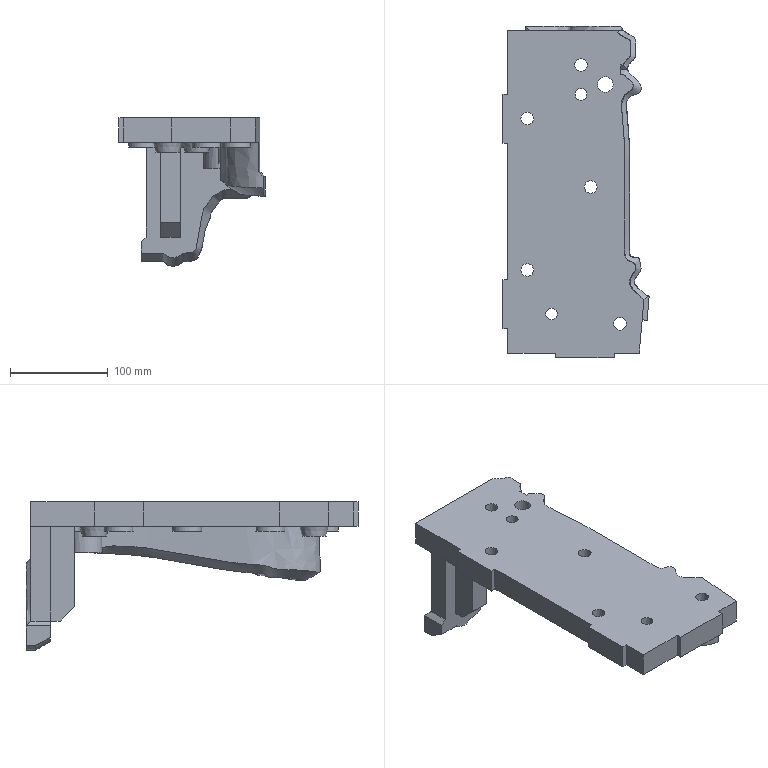Part | NX | features solid 2 | 1 solid | 93 faces | box 149.836 x 340 x 151.908 mm | volume 1528957 mm3 | plane 50 | spline 22 | cylinder 19 | cone 2 | commonest cylinder face diameters 13 x7 30 x4 10 x2 12 x2 32 x2 16 x1